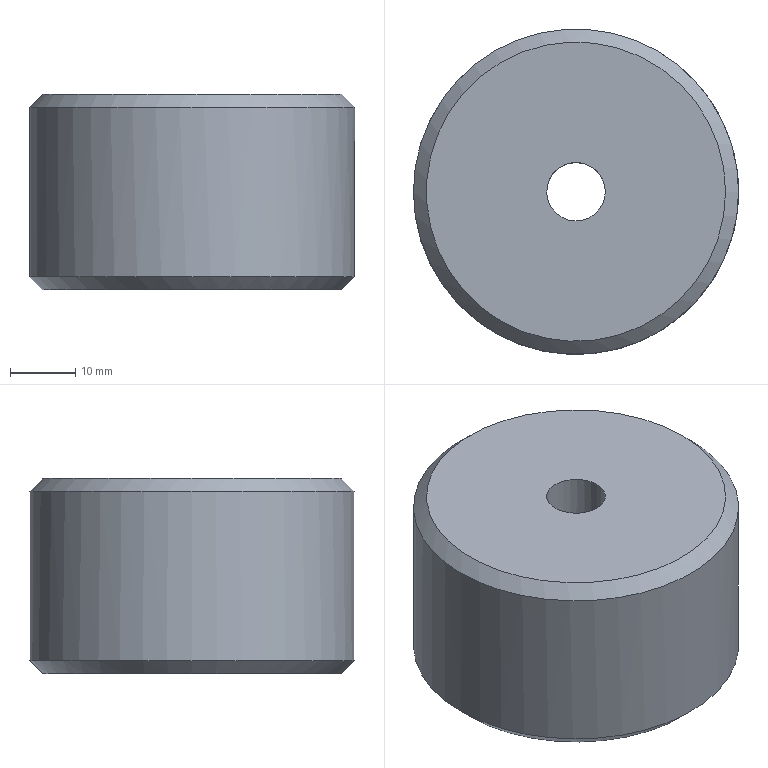Part | STEP file | P011002NM13-000 | 1 solid | 8 faces | box 50 x 50 x 30 mm | volume 55572 mm3 | plane 3 | cylinder 3 | cone 2 | commonest cylinder face diameters 9 x1 14 x1 50 x1
STEP:
#1=CARTESIAN_POINT('',(0.,0.,0.));
#2=DIRECTION('',(0.,0.,1.));
#3=DIRECTION('',(1.,0.,0.));
#4=AXIS2_PLACEMENT_3D('',#1,#2,#3);
#5=CARTESIAN_POINT('',(0.,158.,-181.));
#6=VERTEX_POINT('',#5);
#7=CARTESIAN_POINT('',(0.,165.,-181.));
#8=DIRECTION('',(0.,0.,-1.));
#9=DIRECTION('',(0.,-1.,0.));
#10=AXIS2_PLACEMENT_3D('',#7,#8,#9);
#11=CIRCLE('',#10,7.);
#12=CARTESIAN_POINT('',(0.,165.,-181.));
#13=DIRECTION('',(0.,0.,-1.));
#14=DIRECTION('',(-1.,0.,0.));
#15=AXIS2_PLACEMENT_3D('',#12,#13,#14);
#16=PLANE('',#15);
#17=CARTESIAN_POINT('',(0.,0.));
#18=DIRECTION('',(0.,-1.));
#19=AXIS2_PLACEMENT_2D('',#17,#18);
#20=CIRCLE('',#19,7.);
#21=(GEOMETRIC_REPRESENTATION_CONTEXT(2)PARAMETRIC_REPRESENTATION_CONTEXT()REPRESENTATION_CONTEXT('',''));
#22=DEFINITIONAL_REPRESENTATION('',(#20),#21);
#23=PCURVE('',#16,#22);
#24=CARTESIAN_POINT('',(0.,165.,-182.));
#25=DIRECTION('',(0.,0.,-1.));
#26=DIRECTION('',(0.,-1.,0.));
#27=AXIS2_PLACEMENT_3D('',#24,#25,#26);
#28=CYLINDRICAL_SURFACE('',#27,7.);
#29=CARTESIAN_POINT('',(0.,-1.));
#30=DIRECTION('',(1.,0.));
#31=VECTOR('',#30,1.);
#32=LINE('',#29,#31);
#33=(GEOMETRIC_REPRESENTATION_CONTEXT(2)PARAMETRIC_REPRESENTATION_CONTEXT()REPRESENTATION_CONTEXT('',''));
#34=DEFINITIONAL_REPRESENTATION('',(#32),#33);
#35=PCURVE('',#28,#34);
#36=SURFACE_CURVE('',#11,(#23,#35),.PCURVE_S1.);
#37=EDGE_CURVE('',#6,#6,#36,.T.);
#38=ORIENTED_EDGE('',*,*,#37,.F.);
#39=EDGE_LOOP('',(#38));
#40=FACE_BOUND('',#39,.T.);
#41=CARTESIAN_POINT('',(-23.,165.,-181.));
#42=VERTEX_POINT('',#41);
#43=CARTESIAN_POINT('',(0.,165.,-181.));
#44=DIRECTION('',(0.,0.,-1.));
#45=DIRECTION('',(-1.,0.,0.));
#46=AXIS2_PLACEMENT_3D('',#43,#44,#45);
#47=CIRCLE('',#46,23.);
#48=CARTESIAN_POINT('',(0.,0.));
#49=DIRECTION('',(1.,0.));
#50=AXIS2_PLACEMENT_2D('',#48,#49);
#51=CIRCLE('',#50,23.);
#52=(GEOMETRIC_REPRESENTATION_CONTEXT(2)PARAMETRIC_REPRESENTATION_CONTEXT()REPRESENTATION_CONTEXT('',''));
#53=DEFINITIONAL_REPRESENTATION('',(#51),#52);
#54=PCURVE('',#16,#53);
#55=CARTESIAN_POINT('',(0.,165.,-179.));
#56=DIRECTION('',(0.,0.,1.));
#57=DIRECTION('',(1.,0.,0.));
#58=AXIS2_PLACEMENT_3D('',#55,#56,#57);
#59=CONICAL_SURFACE('',#58,25.,0.7854);
#60=CARTESIAN_POINT('',(9.425,-2.));
#61=DIRECTION('',(-1.,0.));
#62=VECTOR('',#61,1.);
#63=LINE('',#60,#62);
#64=(GEOMETRIC_REPRESENTATION_CONTEXT(2)PARAMETRIC_REPRESENTATION_CONTEXT()REPRESENTATION_CONTEXT('',''));
#65=DEFINITIONAL_REPRESENTATION('',(#63),#64);
#66=PCURVE('',#59,#65);
#67=SURFACE_CURVE('',#47,(#54,#66),.PCURVE_S1.);
#68=EDGE_CURVE('',#42,#42,#67,.T.);
#69=ORIENTED_EDGE('',*,*,#68,.T.);
#70=EDGE_LOOP('',(#69));
#71=FACE_BOUND('',#70,.T.);
#72=ADVANCED_FACE('',(#40,#71),#16,.T.);
#73=CARTESIAN_POINT('',(4.5,165.,-151.));
#74=VERTEX_POINT('',#73);
#75=CARTESIAN_POINT('',(0.,160.5,-151.));
#76=VERTEX_POINT('',#75);
#77=CARTESIAN_POINT('',(0.,165.,-151.));
#78=DIRECTION('',(0.,0.,1.));
#79=DIRECTION('',(1.,0.,0.));
#80=AXIS2_PLACEMENT_3D('',#77,#78,#79);
#81=CIRCLE('',#80,4.5);
#82=CARTESIAN_POINT('',(0.,165.,-151.));
#83=DIRECTION('',(0.,0.,1.));
#84=DIRECTION('',(1.,0.,0.));
#85=AXIS2_PLACEMENT_3D('',#82,#83,#84);
#86=PLANE('',#85);
#87=CARTESIAN_POINT('',(0.,0.));
#88=DIRECTION('',(1.,0.));
#89=AXIS2_PLACEMENT_2D('',#87,#88);
#90=CIRCLE('',#89,4.5);
#91=(GEOMETRIC_REPRESENTATION_CONTEXT(2)PARAMETRIC_REPRESENTATION_CONTEXT()REPRESENTATION_CONTEXT('',''));
#92=DEFINITIONAL_REPRESENTATION('',(#90),#91);
#93=PCURVE('',#86,#92);
#94=CARTESIAN_POINT('',(0.,165.,-182.));
#95=DIRECTION('',(0.,0.,-1.));
#96=DIRECTION('',(0.,-1.,0.));
#97=AXIS2_PLACEMENT_3D('',#94,#95,#96);
#98=CYLINDRICAL_SURFACE('',#97,4.5);
#99=CARTESIAN_POINT('',(4.712,-31.));
#100=DIRECTION('',(-1.,0.));
#101=VECTOR('',#100,1.);
#102=LINE('',#99,#101);
#103=(GEOMETRIC_REPRESENTATION_CONTEXT(2)PARAMETRIC_REPRESENTATION_CONTEXT()REPRESENTATION_CONTEXT('',''));
#104=DEFINITIONAL_REPRESENTATION('',(#102),#103);
#105=PCURVE('',#98,#104);
#106=SURFACE_CURVE('',#81,(#93,#105),.PCURVE_S1.);
#107=EDGE_CURVE('',#74,#76,#106,.T.);
#108=ORIENTED_EDGE('',*,*,#107,.F.);
#109=CARTESIAN_POINT('',(0.,165.,-151.));
#110=DIRECTION('',(0.,0.,1.));
#111=DIRECTION('',(1.,0.,0.));
#112=AXIS2_PLACEMENT_3D('',#109,#110,#111);
#113=CIRCLE('',#112,4.5);
#114=CARTESIAN_POINT('',(0.,0.));
#115=DIRECTION('',(1.,0.));
#116=AXIS2_PLACEMENT_2D('',#114,#115);
#117=CIRCLE('',#116,4.5);
#118=(GEOMETRIC_REPRESENTATION_CONTEXT(2)PARAMETRIC_REPRESENTATION_CONTEXT()REPRESENTATION_CONTEXT('',''));
#119=DEFINITIONAL_REPRESENTATION('',(#117),#118);
#120=PCURVE('',#86,#119);
#121=CARTESIAN_POINT('',(10.996,-31.));
#122=DIRECTION('',(-1.,0.));
#123=VECTOR('',#122,1.);
#124=LINE('',#121,#123);
#125=(GEOMETRIC_REPRESENTATION_CONTEXT(2)PARAMETRIC_REPRESENTATION_CONTEXT()REPRESENTATION_CONTEXT('',''));
#126=DEFINITIONAL_REPRESENTATION('',(#124),#125);
#127=PCURVE('',#98,#126);
#128=SURFACE_CURVE('',#113,(#120,#127),.PCURVE_S1.);
#129=EDGE_CURVE('',#76,#74,#128,.T.);
#130=ORIENTED_EDGE('',*,*,#129,.F.);
#131=EDGE_LOOP('',(#108,#130));
#132=FACE_BOUND('',#131,.T.);
#133=CARTESIAN_POINT('',(23.,165.,-151.));
#134=VERTEX_POINT('',#133);
#135=CARTESIAN_POINT('',(0.,165.,-151.));
#136=DIRECTION('',(0.,0.,1.));
#137=DIRECTION('',(1.,0.,0.));
#138=AXIS2_PLACEMENT_3D('',#135,#136,#137);
#139=CIRCLE('',#138,23.);
#140=CARTESIAN_POINT('',(0.,0.));
#141=DIRECTION('',(1.,0.));
#142=AXIS2_PLACEMENT_2D('',#140,#141);
#143=CIRCLE('',#142,23.);
#144=(GEOMETRIC_REPRESENTATION_CONTEXT(2)PARAMETRIC_REPRESENTATION_CONTEXT()REPRESENTATION_CONTEXT('',''));
#145=DEFINITIONAL_REPRESENTATION('',(#143),#144);
#146=PCURVE('',#86,#145);
#147=CARTESIAN_POINT('',(0.,165.,-153.));
#148=DIRECTION('',(0.,0.,-1.));
#149=DIRECTION('',(-1.,0.,0.));
#150=AXIS2_PLACEMENT_3D('',#147,#148,#149);
#151=CONICAL_SURFACE('',#150,25.,0.7854);
#152=CARTESIAN_POINT('',(9.425,-2.));
#153=DIRECTION('',(-1.,0.));
#154=VECTOR('',#153,1.);
#155=LINE('',#152,#154);
#156=(GEOMETRIC_REPRESENTATION_CONTEXT(2)PARAMETRIC_REPRESENTATION_CONTEXT()REPRESENTATION_CONTEXT('',''));
#157=DEFINITIONAL_REPRESENTATION('',(#155),#156);
#158=PCURVE('',#151,#157);
#159=SURFACE_CURVE('',#139,(#146,#158),.PCURVE_S1.);
#160=EDGE_CURVE('',#134,#134,#159,.T.);
#161=ORIENTED_EDGE('',*,*,#160,.T.);
#162=EDGE_LOOP('',(#161));
#163=FACE_BOUND('',#162,.T.);
#164=ADVANCED_FACE('',(#132,#163),#86,.T.);
#165=CARTESIAN_POINT('',(25.,165.,-153.));
#166=VERTEX_POINT('',#165);
#167=CARTESIAN_POINT('',(-25.,165.,-153.));
#168=VERTEX_POINT('',#167);
#169=CARTESIAN_POINT('',(0.,165.,-153.));
#170=DIRECTION('',(0.,0.,-1.));
#171=DIRECTION('',(1.,0.,0.));
#172=AXIS2_PLACEMENT_3D('',#169,#170,#171);
#173=CIRCLE('',#172,25.);
#174=CARTESIAN_POINT('',(0.,165.,-151.));
#175=DIRECTION('',(0.,0.,-1.));
#176=DIRECTION('',(-1.,0.,0.));
#177=AXIS2_PLACEMENT_3D('',#174,#175,#176);
#178=CYLINDRICAL_SURFACE('',#177,25.);
#179=CARTESIAN_POINT('',(3.142,2.));
#180=DIRECTION('',(1.,0.));
#181=VECTOR('',#180,1.);
#182=LINE('',#179,#181);
#183=(GEOMETRIC_REPRESENTATION_CONTEXT(2)PARAMETRIC_REPRESENTATION_CONTEXT()REPRESENTATION_CONTEXT('',''));
#184=DEFINITIONAL_REPRESENTATION('',(#182),#183);
#185=PCURVE('',#178,#184);
#186=CARTESIAN_POINT('',(3.142,0.));
#187=DIRECTION('',(1.,0.));
#188=VECTOR('',#187,1.);
#189=LINE('',#186,#188);
#190=(GEOMETRIC_REPRESENTATION_CONTEXT(2)PARAMETRIC_REPRESENTATION_CONTEXT()REPRESENTATION_CONTEXT('',''));
#191=DEFINITIONAL_REPRESENTATION('',(#189),#190);
#192=PCURVE('',#151,#191);
#193=SURFACE_CURVE('',#173,(#185,#192),.PCURVE_S1.);
#194=EDGE_CURVE('',#166,#168,#193,.T.);
#195=ORIENTED_EDGE('',*,*,#194,.T.);
#196=CARTESIAN_POINT('',(-25.,165.,-179.));
#197=VERTEX_POINT('',#196);
#198=CARTESIAN_POINT('',(-25.,165.,-153.));
#199=CARTESIAN_POINT('',(-25.,165.,-179.));
#200=B_SPLINE_CURVE_WITH_KNOTS('',1,(#198,#199),.UNSPECIFIED.,.F.,.F.,(2,2),(2.,28.),.PIECEWISE_BEZIER_KNOTS.);
#201=CARTESIAN_POINT('',(6.283,0.));
#202=DIRECTION('',(0.,1.));
#203=VECTOR('',#202,1.);
#204=LINE('',#201,#203);
#205=(GEOMETRIC_REPRESENTATION_CONTEXT(2)PARAMETRIC_REPRESENTATION_CONTEXT()REPRESENTATION_CONTEXT('',''));
#206=DEFINITIONAL_REPRESENTATION('',(#204),#205);
#207=PCURVE('',#178,#206);
#208=CARTESIAN_POINT('',(0.,0.));
#209=DIRECTION('',(0.,1.));
#210=VECTOR('',#209,1.);
#211=LINE('',#208,#210);
#212=(GEOMETRIC_REPRESENTATION_CONTEXT(2)PARAMETRIC_REPRESENTATION_CONTEXT()REPRESENTATION_CONTEXT('',''));
#213=DEFINITIONAL_REPRESENTATION('',(#211),#212);
#214=PCURVE('',#178,#213);
#215=SEAM_CURVE('',#200,(#207,#214),.PCURVE_S1.);
#216=EDGE_CURVE('',#168,#197,#215,.T.);
#217=ORIENTED_EDGE('',*,*,#216,.T.);
#218=CARTESIAN_POINT('',(0.,165.,-179.));
#219=DIRECTION('',(0.,0.,1.));
#220=DIRECTION('',(-1.,0.,0.));
#221=AXIS2_PLACEMENT_3D('',#218,#219,#220);
#222=CIRCLE('',#221,25.);
#223=CARTESIAN_POINT('',(6.283,28.));
#224=DIRECTION('',(-1.,0.));
#225=VECTOR('',#224,1.);
#226=LINE('',#223,#225);
#227=(GEOMETRIC_REPRESENTATION_CONTEXT(2)PARAMETRIC_REPRESENTATION_CONTEXT()REPRESENTATION_CONTEXT('',''));
#228=DEFINITIONAL_REPRESENTATION('',(#226),#227);
#229=PCURVE('',#178,#228);
#230=CARTESIAN_POINT('',(3.142,0.));
#231=DIRECTION('',(1.,0.));
#232=VECTOR('',#231,1.);
#233=LINE('',#230,#232);
#234=(GEOMETRIC_REPRESENTATION_CONTEXT(2)PARAMETRIC_REPRESENTATION_CONTEXT()REPRESENTATION_CONTEXT('',''));
#235=DEFINITIONAL_REPRESENTATION('',(#233),#234);
#236=PCURVE('',#59,#235);
#237=SURFACE_CURVE('',#222,(#229,#236),.PCURVE_S1.);
#238=EDGE_CURVE('',#197,#197,#237,.T.);
#239=ORIENTED_EDGE('',*,*,#238,.T.);
#240=ORIENTED_EDGE('',*,*,#216,.F.);
#241=CARTESIAN_POINT('',(0.,165.,-153.));
#242=DIRECTION('',(0.,0.,-1.));
#243=DIRECTION('',(1.,0.,0.));
#244=AXIS2_PLACEMENT_3D('',#241,#242,#243);
#245=CIRCLE('',#244,25.);
#246=CARTESIAN_POINT('',(-3.142,2.));
#247=DIRECTION('',(1.,0.));
#248=VECTOR('',#247,1.);
#249=LINE('',#246,#248);
#250=(GEOMETRIC_REPRESENTATION_CONTEXT(2)PARAMETRIC_REPRESENTATION_CONTEXT()REPRESENTATION_CONTEXT('',''));
#251=DEFINITIONAL_REPRESENTATION('',(#249),#250);
#252=PCURVE('',#178,#251);
#253=CARTESIAN_POINT('',(3.142,0.));
#254=DIRECTION('',(1.,0.));
#255=VECTOR('',#254,1.);
#256=LINE('',#253,#255);
#257=(GEOMETRIC_REPRESENTATION_CONTEXT(2)PARAMETRIC_REPRESENTATION_CONTEXT()REPRESENTATION_CONTEXT('',''));
#258=DEFINITIONAL_REPRESENTATION('',(#256),#257);
#259=PCURVE('',#151,#258);
#260=SURFACE_CURVE('',#245,(#252,#259),.PCURVE_S1.);
#261=EDGE_CURVE('',#168,#166,#260,.T.);
#262=ORIENTED_EDGE('',*,*,#261,.T.);
#263=EDGE_LOOP('',(#195,#217,#239,#240,#262));
#264=FACE_BOUND('',#263,.T.);
#265=ADVANCED_FACE('',(#264),#178,.T.);
#266=ORIENTED_EDGE('',*,*,#160,.F.);
#267=CARTESIAN_POINT('',(23.,165.,-151.));
#268=CARTESIAN_POINT('',(25.,165.,-153.));
#269=B_SPLINE_CURVE_WITH_KNOTS('',1,(#267,#268),.UNSPECIFIED.,.F.,.F.,(2,2),(-2.828,0.),.PIECEWISE_BEZIER_KNOTS.);
#270=CARTESIAN_POINT('',(9.425,0.));
#271=DIRECTION('',(0.,1.));
#272=VECTOR('',#271,1.);
#273=LINE('',#270,#272);
#274=(GEOMETRIC_REPRESENTATION_CONTEXT(2)PARAMETRIC_REPRESENTATION_CONTEXT()REPRESENTATION_CONTEXT('',''));
#275=DEFINITIONAL_REPRESENTATION('',(#273),#274);
#276=PCURVE('',#151,#275);
#277=CARTESIAN_POINT('',(3.142,0.));
#278=DIRECTION('',(0.,1.));
#279=VECTOR('',#278,1.);
#280=LINE('',#277,#279);
#281=(GEOMETRIC_REPRESENTATION_CONTEXT(2)PARAMETRIC_REPRESENTATION_CONTEXT()REPRESENTATION_CONTEXT('',''));
#282=DEFINITIONAL_REPRESENTATION('',(#280),#281);
#283=PCURVE('',#151,#282);
#284=SEAM_CURVE('',#269,(#276,#283),.PCURVE_S1.);
#285=EDGE_CURVE('',#134,#166,#284,.T.);
#286=ORIENTED_EDGE('',*,*,#285,.T.);
#287=ORIENTED_EDGE('',*,*,#261,.F.);
#288=ORIENTED_EDGE('',*,*,#194,.F.);
#289=ORIENTED_EDGE('',*,*,#285,.F.);
#290=EDGE_LOOP('',(#266,#286,#287,#288,#289));
#291=FACE_BOUND('',#290,.T.);
#292=ADVANCED_FACE('',(#291),#151,.T.);
#293=ORIENTED_EDGE('',*,*,#68,.F.);
#294=CARTESIAN_POINT('',(-23.,165.,-181.));
#295=CARTESIAN_POINT('',(-25.,165.,-179.));
#296=B_SPLINE_CURVE_WITH_KNOTS('',1,(#294,#295),.UNSPECIFIED.,.F.,.F.,(2,2),(-2.828,0.),.PIECEWISE_BEZIER_KNOTS.);
#297=CARTESIAN_POINT('',(9.425,0.));
#298=DIRECTION('',(0.,1.));
#299=VECTOR('',#298,1.);
#300=LINE('',#297,#299);
#301=(GEOMETRIC_REPRESENTATION_CONTEXT(2)PARAMETRIC_REPRESENTATION_CONTEXT()REPRESENTATION_CONTEXT('',''));
#302=DEFINITIONAL_REPRESENTATION('',(#300),#301);
#303=PCURVE('',#59,#302);
#304=CARTESIAN_POINT('',(3.142,0.));
#305=DIRECTION('',(0.,1.));
#306=VECTOR('',#305,1.);
#307=LINE('',#304,#306);
#308=(GEOMETRIC_REPRESENTATION_CONTEXT(2)PARAMETRIC_REPRESENTATION_CONTEXT()REPRESENTATION_CONTEXT('',''));
#309=DEFINITIONAL_REPRESENTATION('',(#307),#308);
#310=PCURVE('',#59,#309);
#311=SEAM_CURVE('',#296,(#303,#310),.PCURVE_S1.);
#312=EDGE_CURVE('',#42,#197,#311,.T.);
#313=ORIENTED_EDGE('',*,*,#312,.T.);
#314=ORIENTED_EDGE('',*,*,#238,.F.);
#315=ORIENTED_EDGE('',*,*,#312,.F.);
#316=EDGE_LOOP('',(#293,#313,#314,#315));
#317=FACE_BOUND('',#316,.T.);
#318=ADVANCED_FACE('',(#317),#59,.T.);
#319=ORIENTED_EDGE('',*,*,#129,.F.);
#320=CARTESIAN_POINT('',(0.,160.5,-172.));
#321=VERTEX_POINT('',#320);
#322=CARTESIAN_POINT('',(0.,160.5,-151.));
#323=CARTESIAN_POINT('',(0.,160.5,-172.));
#324=B_SPLINE_CURVE_WITH_KNOTS('',1,(#322,#323),.UNSPECIFIED.,.F.,.F.,(2,2),(-31.,-10.),.PIECEWISE_BEZIER_KNOTS.);
#325=CARTESIAN_POINT('',(6.283,0.));
#326=DIRECTION('',(0.,1.));
#327=VECTOR('',#326,1.);
#328=LINE('',#325,#327);
#329=(GEOMETRIC_REPRESENTATION_CONTEXT(2)PARAMETRIC_REPRESENTATION_CONTEXT()REPRESENTATION_CONTEXT('',''));
#330=DEFINITIONAL_REPRESENTATION('',(#328),#329);
#331=PCURVE('',#98,#330);
#332=CARTESIAN_POINT('',(0.,0.));
#333=DIRECTION('',(0.,1.));
#334=VECTOR('',#333,1.);
#335=LINE('',#332,#334);
#336=(GEOMETRIC_REPRESENTATION_CONTEXT(2)PARAMETRIC_REPRESENTATION_CONTEXT()REPRESENTATION_CONTEXT('',''));
#337=DEFINITIONAL_REPRESENTATION('',(#335),#336);
#338=PCURVE('',#98,#337);
#339=SEAM_CURVE('',#324,(#331,#338),.PCURVE_S1.);
#340=EDGE_CURVE('',#76,#321,#339,.T.);
#341=ORIENTED_EDGE('',*,*,#340,.T.);
#342=CARTESIAN_POINT('',(0.,165.,-172.));
#343=DIRECTION('',(0.,0.,-1.));
#344=DIRECTION('',(0.,-1.,0.));
#345=AXIS2_PLACEMENT_3D('',#342,#343,#344);
#346=CIRCLE('',#345,4.5);
#347=CARTESIAN_POINT('',(0.,-10.));
#348=DIRECTION('',(1.,0.));
#349=VECTOR('',#348,1.);
#350=LINE('',#347,#349);
#351=(GEOMETRIC_REPRESENTATION_CONTEXT(2)PARAMETRIC_REPRESENTATION_CONTEXT()REPRESENTATION_CONTEXT('',''));
#352=DEFINITIONAL_REPRESENTATION('',(#350),#351);
#353=PCURVE('',#98,#352);
#354=CARTESIAN_POINT('',(0.,165.,-172.));
#355=DIRECTION('',(0.,0.,-1.));
#356=DIRECTION('',(0.,-1.,0.));
#357=AXIS2_PLACEMENT_3D('',#354,#355,#356);
#358=PLANE('',#357);
#359=CARTESIAN_POINT('',(0.,0.));
#360=DIRECTION('',(1.,0.));
#361=AXIS2_PLACEMENT_2D('',#359,#360);
#362=CIRCLE('',#361,4.5);
#363=(GEOMETRIC_REPRESENTATION_CONTEXT(2)PARAMETRIC_REPRESENTATION_CONTEXT()REPRESENTATION_CONTEXT('',''));
#364=DEFINITIONAL_REPRESENTATION('',(#362),#363);
#365=PCURVE('',#358,#364);
#366=SURFACE_CURVE('',#346,(#353,#365),.PCURVE_S1.);
#367=EDGE_CURVE('',#321,#321,#366,.T.);
#368=ORIENTED_EDGE('',*,*,#367,.F.);
#369=ORIENTED_EDGE('',*,*,#340,.F.);
#370=ORIENTED_EDGE('',*,*,#107,.F.);
#371=EDGE_LOOP('',(#319,#341,#368,#369,#370));
#372=FACE_BOUND('',#371,.F.);
#373=ADVANCED_FACE('',(#372),#98,.F.);
#374=ORIENTED_EDGE('',*,*,#367,.F.);
#375=EDGE_LOOP('',(#374));
#376=FACE_BOUND('',#375,.T.);
#377=CARTESIAN_POINT('',(0.,158.,-172.));
#378=VERTEX_POINT('',#377);
#379=CARTESIAN_POINT('',(0.,165.,-172.));
#380=DIRECTION('',(0.,0.,-1.));
#381=DIRECTION('',(0.,-1.,0.));
#382=AXIS2_PLACEMENT_3D('',#379,#380,#381);
#383=CIRCLE('',#382,7.);
#384=CARTESIAN_POINT('',(0.,0.));
#385=DIRECTION('',(1.,0.));
#386=AXIS2_PLACEMENT_2D('',#384,#385);
#387=CIRCLE('',#386,7.);
#388=(GEOMETRIC_REPRESENTATION_CONTEXT(2)PARAMETRIC_REPRESENTATION_CONTEXT()REPRESENTATION_CONTEXT('',''));
#389=DEFINITIONAL_REPRESENTATION('',(#387),#388);
#390=PCURVE('',#358,#389);
#391=CARTESIAN_POINT('',(0.,-10.));
#392=DIRECTION('',(1.,0.));
#393=VECTOR('',#392,1.);
#394=LINE('',#391,#393);
#395=(GEOMETRIC_REPRESENTATION_CONTEXT(2)PARAMETRIC_REPRESENTATION_CONTEXT()REPRESENTATION_CONTEXT('',''));
#396=DEFINITIONAL_REPRESENTATION('',(#394),#395);
#397=PCURVE('',#28,#396);
#398=SURFACE_CURVE('',#383,(#390,#397),.PCURVE_S1.);
#399=EDGE_CURVE('',#378,#378,#398,.T.);
#400=ORIENTED_EDGE('',*,*,#399,.T.);
#401=EDGE_LOOP('',(#400));
#402=FACE_BOUND('',#401,.T.);
#403=ADVANCED_FACE('',(#376,#402),#358,.T.);
#404=ORIENTED_EDGE('',*,*,#37,.F.);
#405=CARTESIAN_POINT('',(0.,158.,-172.));
#406=CARTESIAN_POINT('',(0.,158.,-181.));
#407=B_SPLINE_CURVE_WITH_KNOTS('',1,(#405,#406),.UNSPECIFIED.,.F.,.F.,(2,2),(-10.,-1.),.PIECEWISE_BEZIER_KNOTS.);
#408=CARTESIAN_POINT('',(0.,0.));
#409=DIRECTION('',(0.,1.));
#410=VECTOR('',#409,1.);
#411=LINE('',#408,#410);
#412=(GEOMETRIC_REPRESENTATION_CONTEXT(2)PARAMETRIC_REPRESENTATION_CONTEXT()REPRESENTATION_CONTEXT('',''));
#413=DEFINITIONAL_REPRESENTATION('',(#411),#412);
#414=PCURVE('',#28,#413);
#415=CARTESIAN_POINT('',(6.283,0.));
#416=DIRECTION('',(0.,1.));
#417=VECTOR('',#416,1.);
#418=LINE('',#415,#417);
#419=(GEOMETRIC_REPRESENTATION_CONTEXT(2)PARAMETRIC_REPRESENTATION_CONTEXT()REPRESENTATION_CONTEXT('',''));
#420=DEFINITIONAL_REPRESENTATION('',(#418),#419);
#421=PCURVE('',#28,#420);
#422=SEAM_CURVE('',#407,(#414,#421),.PCURVE_S1.);
#423=EDGE_CURVE('',#378,#6,#422,.T.);
#424=ORIENTED_EDGE('',*,*,#423,.F.);
#425=ORIENTED_EDGE('',*,*,#399,.T.);
#426=ORIENTED_EDGE('',*,*,#423,.T.);
#427=EDGE_LOOP('',(#404,#424,#425,#426));
#428=FACE_BOUND('',#427,.F.);
#429=ADVANCED_FACE('',(#428),#28,.F.);
#430=CLOSED_SHELL('',(#72,#164,#265,#292,#318,#373,#403,#429));
#431=MANIFOLD_SOLID_BREP('',#430);
#432=(LENGTH_UNIT()NAMED_UNIT(*)SI_UNIT(.MILLI.,.METRE.));
#433=UNCERTAINTY_MEASURE_WITH_UNIT(LENGTH_MEASURE(0.00001),#432,'','');
#434=(NAMED_UNIT(*)PLANE_ANGLE_UNIT()SI_UNIT($,.RADIAN.));
#435=(NAMED_UNIT(*)SI_UNIT($,.STERADIAN.)SOLID_ANGLE_UNIT());
#436=(GEOMETRIC_REPRESENTATION_CONTEXT(3)GLOBAL_UNCERTAINTY_ASSIGNED_CONTEXT((#433))GLOBAL_UNIT_ASSIGNED_CONTEXT((#432,#434,#435))REPRESENTATION_CONTEXT('',''));
#437=ADVANCED_BREP_SHAPE_REPRESENTATION('',(#4,#431),#436);